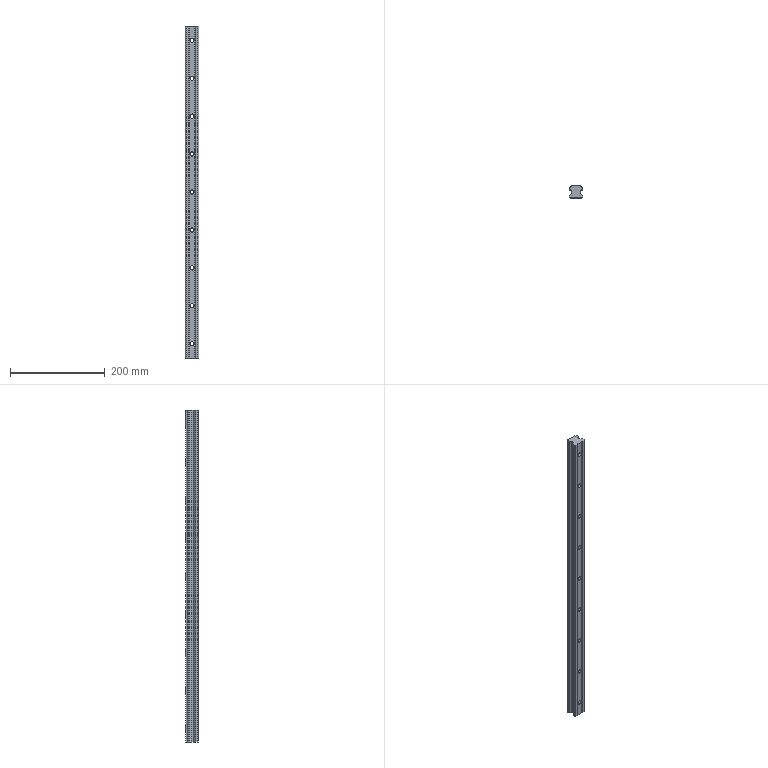Part | SolidWorks | features ICE 8, Draft 4, Fillet 2, Chamfer 1, Extrusion 1, HoleWzd 1 | 1 solid | 97 faces | box 28 x 26 x 700 mm | volume 404636 mm3 | cylinder 58 | plane 39 | commonest cylinder face diameters 9 x18 14 x18 1.2 x12 1.6 x6 5.66 x4